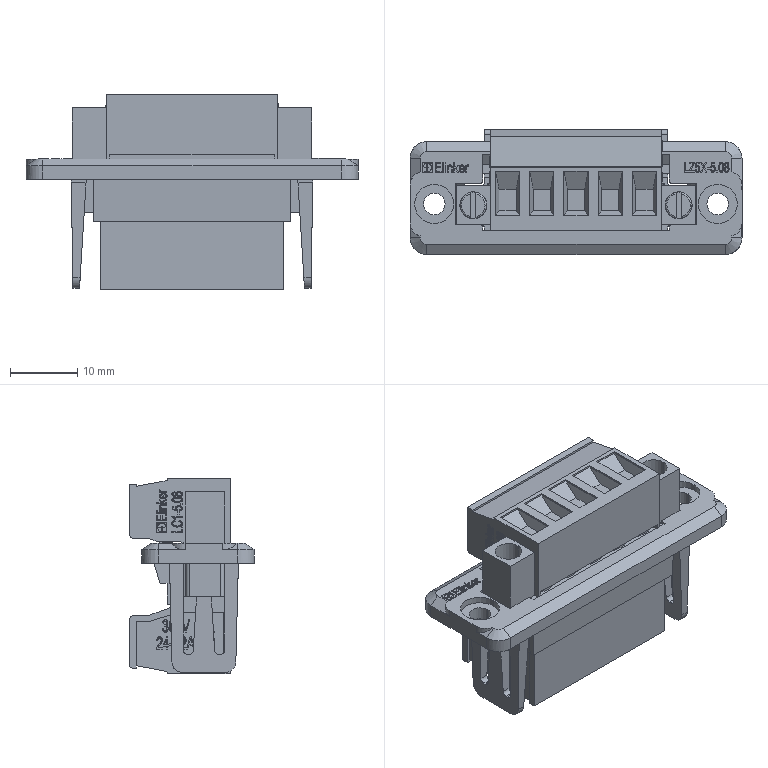Part | NX | features BREP 24 | 24 solids | 7722 faces | volume 11022 mm3 | plane 6947 | cylinder 332 | spline 302 | torus 104 | cone 37 | commonest cylinder face diameters 3.2 x48 3.6 x36 3.9 x24 4 x24 2.5 x22 1.2 x12